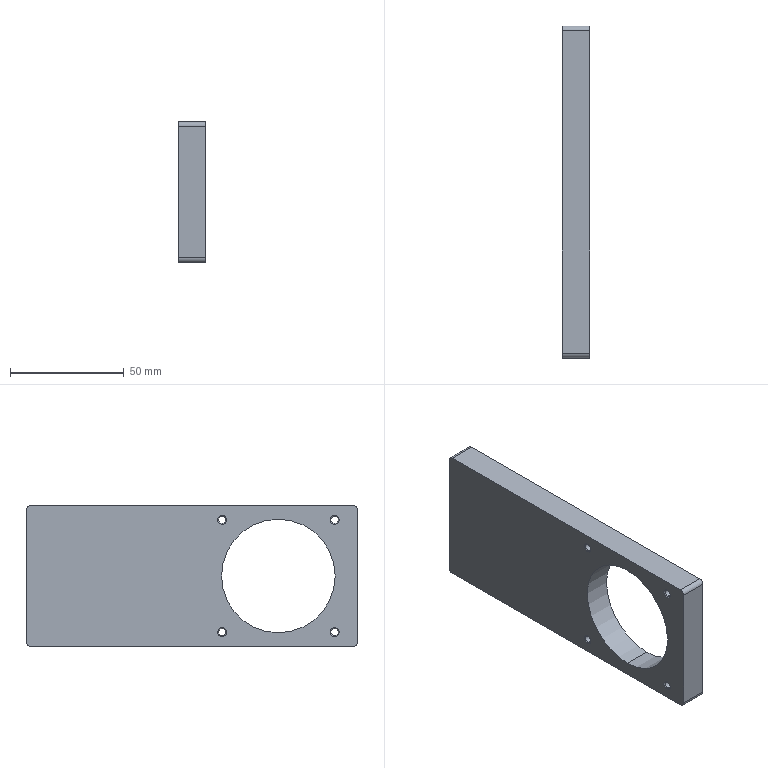Part | STEP file | 1 solid | 36 faces | box 12 x 146 x 62 mm | volume 84618 mm3 | cone 16 | cylinder 14 | plane 6 | commonest cylinder face diameters 3.242 x8 4 x4 50 x2